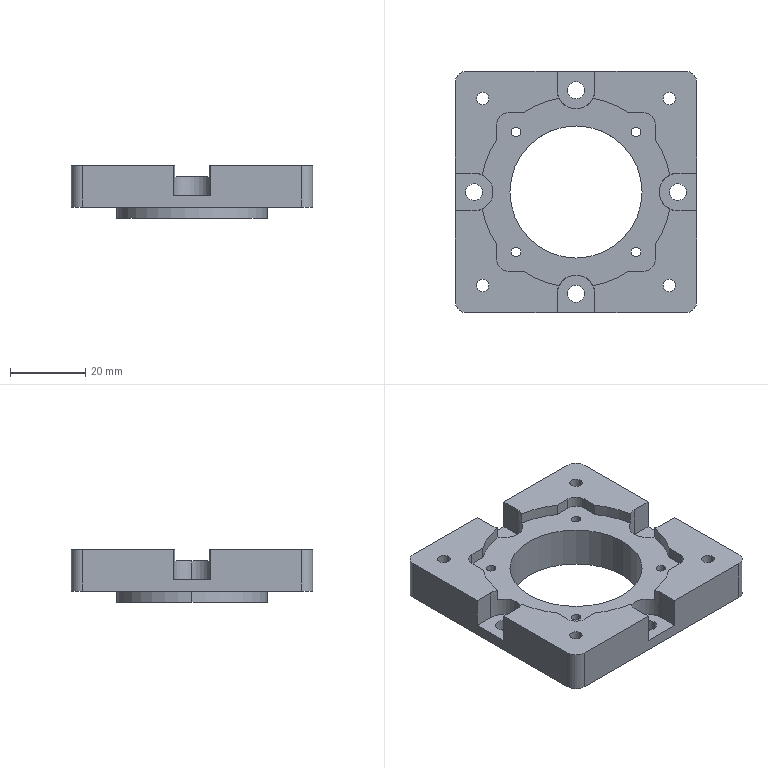Part | SolidWorks | features BaseBody 1 | 1 solid | 80 faces | box 64 x 64 x 14 mm | volume 28587 mm3 | cylinder 49 | plane 31 | commonest cylinder face diameters 2.5 x8 3.3 x8 4.5 x8 6 x8 50.5 x8 10 x5